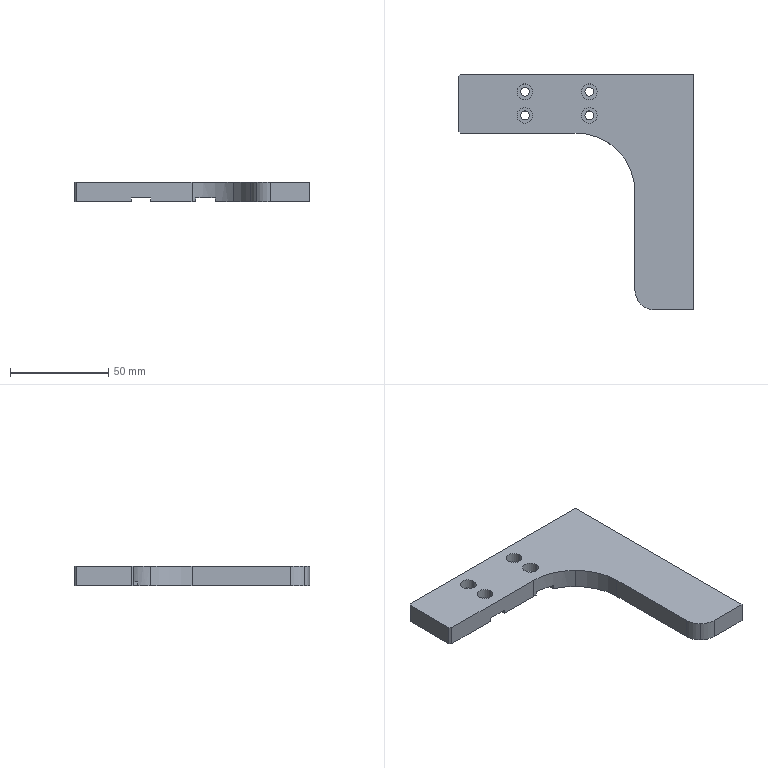Part | STEP file | ASND-0110-Body 1-16 | 1 solid | 54 faces | box 120 x 120 x 10 mm | volume 61912 mm3 | cylinder 26 | plane 22 | cone 6 | commonest cylinder face diameters 4.5 x8 8 x8 3.242 x6 20 x2 60 x2